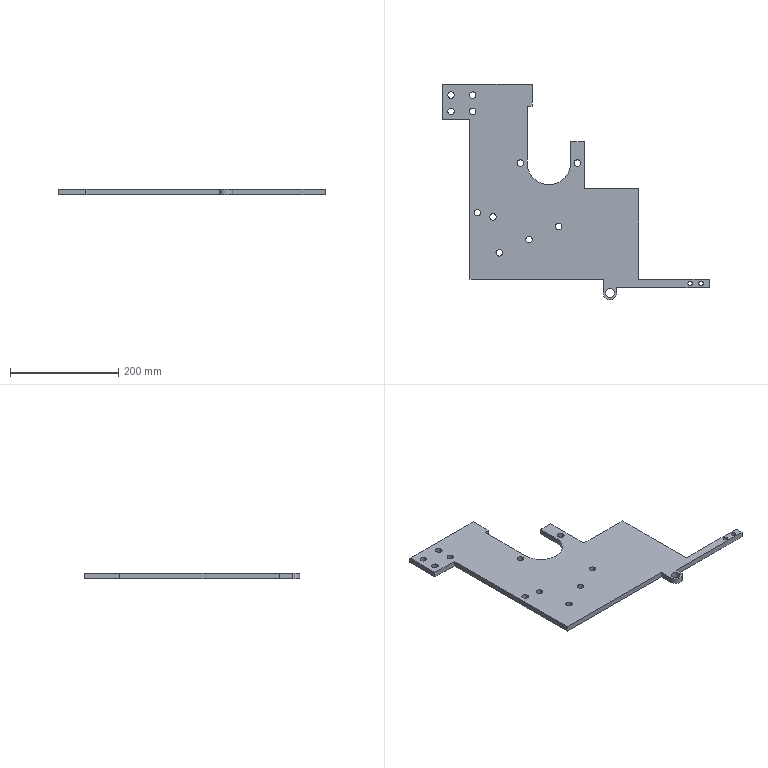Part | SolidWorks | features ICE 5, Cut 1, Extrusion 1 | 1 solid | 50 faces | box 490.997 x 397.445 x 10 mm | volume 813417 mm3 | cylinder 30 | plane 20 | commonest cylinder face diameters 12 x22 8 x4 16 x2 25 x1 80 x1